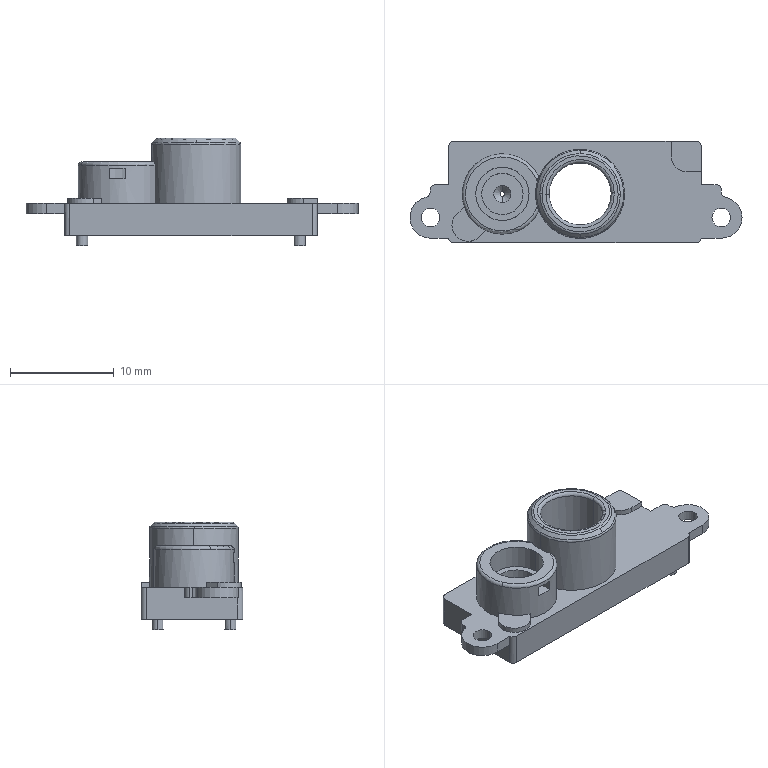Part | SolidWorks | features BaseBody 1 | 1 solid | 95 faces | box 32.054 x 9.8 x 10.4 mm | volume 740.957 mm3 | plane 46 | cylinder 36 | torus 9 | cone 4 | commonest cylinder face diameters 1 x8 4 x5 1.1 x4 1.2 x4 1.8 x4 3.15 x4